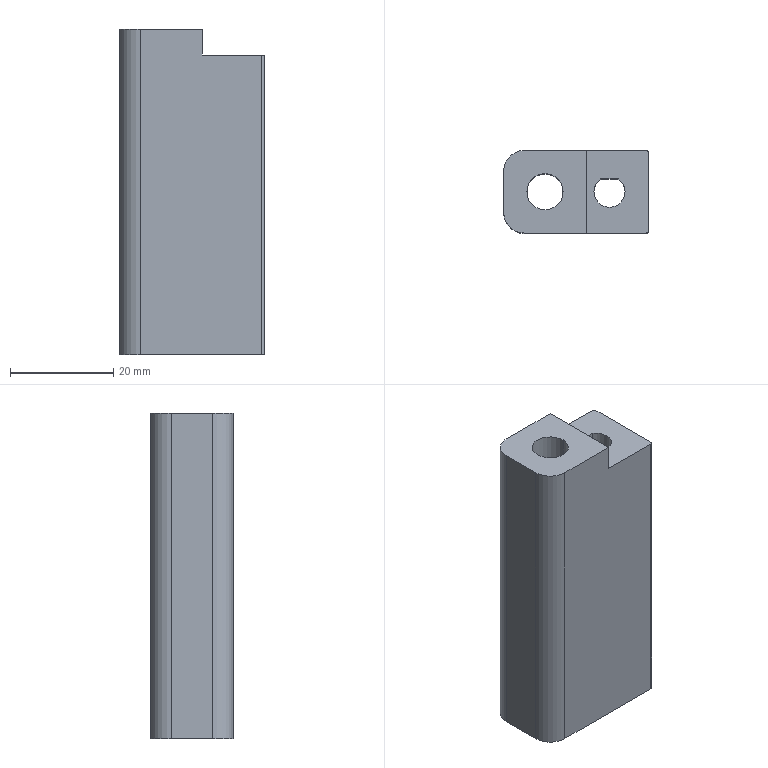Part | 1 solid | 19 faces | box 28 x 16 x 63 mm | volume 22260 mm3 | plane 10 | cylinder 9 | commonest cylinder face diameters 1 x2 7 x2 8 x2 11 x2 6 x1
STEP:
#1=CARTESIAN_POINT('',(0.,0.,0.));
#2=DIRECTION('',(0.,0.,1.));
#3=DIRECTION('',(1.,0.,0.));
#4=AXIS2_PLACEMENT_3D('',#1,#2,#3);
#5=CARTESIAN_POINT('',(-264.863,475.5,-113.051));
#6=VERTEX_POINT('',#5);
#7=CARTESIAN_POINT('',(-271.863,475.5,-113.051));
#8=VERTEX_POINT('',#7);
#9=CARTESIAN_POINT('',(-268.363,475.5,-113.051));
#10=DIRECTION('',(0.,0.,1.));
#11=DIRECTION('',(-1.,0.,0.));
#12=AXIS2_PLACEMENT_3D('',#9,#10,#11);
#13=CIRCLE('',#12,3.5);
#14=CARTESIAN_POINT('',(-248.863,468.,-113.051));
#15=DIRECTION('',(0.,0.,-1.));
#16=DIRECTION('',(1.,0.,0.));
#17=AXIS2_PLACEMENT_3D('',#14,#15,#16);
#18=PLANE('',#17);
#19=CARTESIAN_POINT('',(-23.,-7.5));
#20=CARTESIAN_POINT('',(-23.,-1.438));
#21=CARTESIAN_POINT('',(-17.75,-4.469));
#22=CARTESIAN_POINT('',(-12.5,-7.5));
#23=CARTESIAN_POINT('',(-17.75,-10.531));
#24=CARTESIAN_POINT('',(-23.,-13.562));
#25=CARTESIAN_POINT('',(-23.,-7.5));
#26=(BOUNDED_CURVE()B_SPLINE_CURVE(2,(#19,#20,#21,#22,#23,#24,#25),.UNSPECIFIED.,.T.,.F.)B_SPLINE_CURVE_WITH_KNOTS((1,2,2,2,2,1),(-2.094,0.,2.094,4.189,6.283,8.378),.UNSPECIFIED.)CURVE()GEOMETRIC_REPRESENTATION_ITEM()RATIONAL_B_SPLINE_CURVE((1.,0.5,1.,0.5,1.,0.5,1.))REPRESENTATION_ITEM(''));
#27=(GEOMETRIC_REPRESENTATION_CONTEXT(2)PARAMETRIC_REPRESENTATION_CONTEXT()REPRESENTATION_CONTEXT('',''));
#28=DEFINITIONAL_REPRESENTATION('',(#26),#27);
#29=PCURVE('',#18,#28);
#30=CARTESIAN_POINT('',(-268.363,475.5,-149.051));
#31=DIRECTION('',(0.,0.,1.));
#32=DIRECTION('',(0.,-1.,0.));
#33=AXIS2_PLACEMENT_3D('',#30,#31,#32);
#34=CYLINDRICAL_SURFACE('',#33,3.5);
#35=CARTESIAN_POINT('',(-1.571,36.));
#36=DIRECTION('',(1.,0.));
#37=VECTOR('',#36,1.);
#38=LINE('',#35,#37);
#39=(GEOMETRIC_REPRESENTATION_CONTEXT(2)PARAMETRIC_REPRESENTATION_CONTEXT()REPRESENTATION_CONTEXT('',''));
#40=DEFINITIONAL_REPRESENTATION('',(#38),#39);
#41=PCURVE('',#34,#40);
#42=SURFACE_CURVE('',#13,(#29,#41),.PCURVE_S1.);
#43=EDGE_CURVE('',#6,#8,#42,.T.);
#44=ORIENTED_EDGE('',*,*,#43,.F.);
#45=CARTESIAN_POINT('',(-268.363,475.5,-113.051));
#46=DIRECTION('',(0.,0.,1.));
#47=DIRECTION('',(-1.,0.,0.));
#48=AXIS2_PLACEMENT_3D('',#45,#46,#47);
#49=CIRCLE('',#48,3.5);
#50=CARTESIAN_POINT('',(-23.,-7.5));
#51=CARTESIAN_POINT('',(-23.,-1.438));
#52=CARTESIAN_POINT('',(-17.75,-4.469));
#53=CARTESIAN_POINT('',(-12.5,-7.5));
#54=CARTESIAN_POINT('',(-17.75,-10.531));
#55=CARTESIAN_POINT('',(-23.,-13.562));
#56=CARTESIAN_POINT('',(-23.,-7.5));
#57=(BOUNDED_CURVE()B_SPLINE_CURVE(2,(#50,#51,#52,#53,#54,#55,#56),.UNSPECIFIED.,.T.,.F.)B_SPLINE_CURVE_WITH_KNOTS((1,2,2,2,2,1),(-2.094,0.,2.094,4.189,6.283,8.378),.UNSPECIFIED.)CURVE()GEOMETRIC_REPRESENTATION_ITEM()RATIONAL_B_SPLINE_CURVE((1.,0.5,1.,0.5,1.,0.5,1.))REPRESENTATION_ITEM(''));
#58=(GEOMETRIC_REPRESENTATION_CONTEXT(2)PARAMETRIC_REPRESENTATION_CONTEXT()REPRESENTATION_CONTEXT('',''));
#59=DEFINITIONAL_REPRESENTATION('',(#57),#58);
#60=PCURVE('',#18,#59);
#61=CARTESIAN_POINT('',(-268.363,475.5,-149.051));
#62=DIRECTION('',(0.,0.,1.));
#63=DIRECTION('',(0.,1.,0.));
#64=AXIS2_PLACEMENT_3D('',#61,#62,#63);
#65=CYLINDRICAL_SURFACE('',#64,3.5);
#66=CARTESIAN_POINT('',(1.571,36.));
#67=DIRECTION('',(1.,0.));
#68=VECTOR('',#67,1.);
#69=LINE('',#66,#68);
#70=(GEOMETRIC_REPRESENTATION_CONTEXT(2)PARAMETRIC_REPRESENTATION_CONTEXT()REPRESENTATION_CONTEXT('',''));
#71=DEFINITIONAL_REPRESENTATION('',(#69),#70);
#72=PCURVE('',#65,#71);
#73=SURFACE_CURVE('',#49,(#60,#72),.PCURVE_S1.);
#74=EDGE_CURVE('',#8,#6,#73,.T.);
#75=ORIENTED_EDGE('',*,*,#74,.F.);
#76=EDGE_LOOP('',(#44,#75));
#77=FACE_BOUND('',#76,.T.);
#78=CARTESIAN_POINT('',(-260.363,483.5,-113.051));
#79=VERTEX_POINT('',#78);
#80=CARTESIAN_POINT('',(-260.363,467.5,-113.051));
#81=VERTEX_POINT('',#80);
#82=CARTESIAN_POINT('',(-260.363,468.,-113.051));
#83=DIRECTION('',(0.,-1.,0.));
#84=VECTOR('',#83,1.);
#85=LINE('',#82,#84);
#86=CARTESIAN_POINT('',(-11.5,0.));
#87=DIRECTION('',(0.,1.));
#88=VECTOR('',#87,1.);
#89=LINE('',#86,#88);
#90=(GEOMETRIC_REPRESENTATION_CONTEXT(2)PARAMETRIC_REPRESENTATION_CONTEXT()REPRESENTATION_CONTEXT('',''));
#91=DEFINITIONAL_REPRESENTATION('',(#89),#90);
#92=PCURVE('',#18,#91);
#93=CARTESIAN_POINT('',(-260.363,483.,-108.051));
#94=DIRECTION('',(1.,0.,0.));
#95=DIRECTION('',(0.,0.,1.));
#96=AXIS2_PLACEMENT_3D('',#93,#94,#95);
#97=PLANE('',#96);
#98=CARTESIAN_POINT('',(-5.,15.));
#99=DIRECTION('',(0.,1.));
#100=VECTOR('',#99,1.);
#101=LINE('',#98,#100);
#102=(GEOMETRIC_REPRESENTATION_CONTEXT(2)PARAMETRIC_REPRESENTATION_CONTEXT()REPRESENTATION_CONTEXT('',''));
#103=DEFINITIONAL_REPRESENTATION('',(#101),#102);
#104=PCURVE('',#97,#103);
#105=SURFACE_CURVE('',#85,(#92,#104),.PCURVE_S1.);
#106=EDGE_CURVE('',#79,#81,#105,.T.);
#107=ORIENTED_EDGE('',*,*,#106,.F.);
#108=CARTESIAN_POINT('',(-272.363,483.5,-113.051));
#109=VERTEX_POINT('',#108);
#110=CARTESIAN_POINT('',(-272.363,483.5,-113.051));
#111=DIRECTION('',(1.,0.,0.));
#112=VECTOR('',#111,1.);
#113=LINE('',#110,#112);
#114=CARTESIAN_POINT('',(-23.5,-15.5));
#115=DIRECTION('',(1.,0.));
#116=VECTOR('',#115,1.);
#117=LINE('',#114,#116);
#118=(GEOMETRIC_REPRESENTATION_CONTEXT(2)PARAMETRIC_REPRESENTATION_CONTEXT()REPRESENTATION_CONTEXT('',''));
#119=DEFINITIONAL_REPRESENTATION('',(#117),#118);
#120=PCURVE('',#18,#119);
#121=CARTESIAN_POINT('',(-272.363,483.5,-149.051));
#122=DIRECTION('',(0.,-1.,0.));
#123=DIRECTION('',(-1.,0.,0.));
#124=AXIS2_PLACEMENT_3D('',#121,#122,#123);
#125=PLANE('',#124);
#126=CARTESIAN_POINT('',(0.,-36.));
#127=DIRECTION('',(-1.,0.));
#128=VECTOR('',#127,1.);
#129=LINE('',#126,#128);
#130=(GEOMETRIC_REPRESENTATION_CONTEXT(2)PARAMETRIC_REPRESENTATION_CONTEXT()REPRESENTATION_CONTEXT('',''));
#131=DEFINITIONAL_REPRESENTATION('',(#129),#130);
#132=PCURVE('',#125,#131);
#133=SURFACE_CURVE('',#113,(#120,#132),.PCURVE_S1.);
#134=EDGE_CURVE('',#109,#79,#133,.T.);
#135=ORIENTED_EDGE('',*,*,#134,.F.);
#136=CARTESIAN_POINT('',(-276.363,479.5,-113.051));
#137=VERTEX_POINT('',#136);
#138=CARTESIAN_POINT('',(-272.363,479.5,-113.051));
#139=DIRECTION('',(0.,0.,-1.));
#140=DIRECTION('',(1.,0.,0.));
#141=AXIS2_PLACEMENT_3D('',#138,#139,#140);
#142=CIRCLE('',#141,4.);
#143=CARTESIAN_POINT('',(-23.5,-11.5));
#144=DIRECTION('',(1.,0.));
#145=AXIS2_PLACEMENT_2D('',#143,#144);
#146=CIRCLE('',#145,4.);
#147=(GEOMETRIC_REPRESENTATION_CONTEXT(2)PARAMETRIC_REPRESENTATION_CONTEXT()REPRESENTATION_CONTEXT('',''));
#148=DEFINITIONAL_REPRESENTATION('',(#146),#147);
#149=PCURVE('',#18,#148);
#150=CARTESIAN_POINT('',(-272.363,479.5,-149.051));
#151=DIRECTION('',(0.,0.,1.));
#152=DIRECTION('',(0.7071,-0.7071,0.));
#153=AXIS2_PLACEMENT_3D('',#150,#151,#152);
#154=CYLINDRICAL_SURFACE('',#153,4.);
#155=CARTESIAN_POINT('',(7.069,36.));
#156=DIRECTION('',(-1.,0.));
#157=VECTOR('',#156,1.);
#158=LINE('',#155,#157);
#159=(GEOMETRIC_REPRESENTATION_CONTEXT(2)PARAMETRIC_REPRESENTATION_CONTEXT()REPRESENTATION_CONTEXT('',''));
#160=DEFINITIONAL_REPRESENTATION('',(#158),#159);
#161=PCURVE('',#154,#160);
#162=SURFACE_CURVE('',#142,(#149,#161),.PCURVE_S1.);
#163=EDGE_CURVE('',#137,#109,#162,.T.);
#164=ORIENTED_EDGE('',*,*,#163,.F.);
#165=CARTESIAN_POINT('',(-276.363,471.5,-113.051));
#166=VERTEX_POINT('',#165);
#167=CARTESIAN_POINT('',(-276.363,471.5,-113.051));
#168=DIRECTION('',(0.,1.,0.));
#169=VECTOR('',#168,1.);
#170=LINE('',#167,#169);
#171=CARTESIAN_POINT('',(-27.5,-3.5));
#172=DIRECTION('',(0.,-1.));
#173=VECTOR('',#172,1.);
#174=LINE('',#171,#173);
#175=(GEOMETRIC_REPRESENTATION_CONTEXT(2)PARAMETRIC_REPRESENTATION_CONTEXT()REPRESENTATION_CONTEXT('',''));
#176=DEFINITIONAL_REPRESENTATION('',(#174),#175);
#177=PCURVE('',#18,#176);
#178=CARTESIAN_POINT('',(-276.363,471.5,-149.051));
#179=DIRECTION('',(1.,0.,0.));
#180=DIRECTION('',(0.,-1.,0.));
#181=AXIS2_PLACEMENT_3D('',#178,#179,#180);
#182=PLANE('',#181);
#183=CARTESIAN_POINT('',(0.,-36.));
#184=DIRECTION('',(-1.,0.));
#185=VECTOR('',#184,1.);
#186=LINE('',#183,#185);
#187=(GEOMETRIC_REPRESENTATION_CONTEXT(2)PARAMETRIC_REPRESENTATION_CONTEXT()REPRESENTATION_CONTEXT('',''));
#188=DEFINITIONAL_REPRESENTATION('',(#186),#187);
#189=PCURVE('',#182,#188);
#190=SURFACE_CURVE('',#170,(#177,#189),.PCURVE_S1.);
#191=EDGE_CURVE('',#166,#137,#190,.T.);
#192=ORIENTED_EDGE('',*,*,#191,.F.);
#193=CARTESIAN_POINT('',(-272.363,467.5,-113.051));
#194=VERTEX_POINT('',#193);
#195=CARTESIAN_POINT('',(-272.363,471.5,-113.051));
#196=DIRECTION('',(0.,0.,-1.));
#197=DIRECTION('',(1.,0.,0.));
#198=AXIS2_PLACEMENT_3D('',#195,#196,#197);
#199=CIRCLE('',#198,4.);
#200=CARTESIAN_POINT('',(-23.5,-3.5));
#201=DIRECTION('',(1.,0.));
#202=AXIS2_PLACEMENT_2D('',#200,#201);
#203=CIRCLE('',#202,4.);
#204=(GEOMETRIC_REPRESENTATION_CONTEXT(2)PARAMETRIC_REPRESENTATION_CONTEXT()REPRESENTATION_CONTEXT('',''));
#205=DEFINITIONAL_REPRESENTATION('',(#203),#204);
#206=PCURVE('',#18,#205);
#207=CARTESIAN_POINT('',(-272.363,471.5,-149.051));
#208=DIRECTION('',(0.,0.,1.));
#209=DIRECTION('',(0.7071,0.7071,0.));
#210=AXIS2_PLACEMENT_3D('',#207,#208,#209);
#211=CYLINDRICAL_SURFACE('',#210,4.);
#212=CARTESIAN_POINT('',(5.498,36.));
#213=DIRECTION('',(-1.,0.));
#214=VECTOR('',#213,1.);
#215=LINE('',#212,#214);
#216=(GEOMETRIC_REPRESENTATION_CONTEXT(2)PARAMETRIC_REPRESENTATION_CONTEXT()REPRESENTATION_CONTEXT('',''));
#217=DEFINITIONAL_REPRESENTATION('',(#215),#216);
#218=PCURVE('',#211,#217);
#219=SURFACE_CURVE('',#199,(#206,#218),.PCURVE_S1.);
#220=EDGE_CURVE('',#194,#166,#219,.T.);
#221=ORIENTED_EDGE('',*,*,#220,.F.);
#222=CARTESIAN_POINT('',(-248.863,467.5,-113.051));
#223=DIRECTION('',(-1.,0.,0.));
#224=VECTOR('',#223,1.);
#225=LINE('',#222,#224);
#226=CARTESIAN_POINT('',(0.,0.5));
#227=DIRECTION('',(-1.,0.));
#228=VECTOR('',#227,1.);
#229=LINE('',#226,#228);
#230=(GEOMETRIC_REPRESENTATION_CONTEXT(2)PARAMETRIC_REPRESENTATION_CONTEXT()REPRESENTATION_CONTEXT('',''));
#231=DEFINITIONAL_REPRESENTATION('',(#229),#230);
#232=PCURVE('',#18,#231);
#233=CARTESIAN_POINT('',(-248.863,467.5,-149.051));
#234=DIRECTION('',(0.,1.,0.));
#235=DIRECTION('',(0.,0.,-1.));
#236=AXIS2_PLACEMENT_3D('',#233,#234,#235);
#237=PLANE('',#236);
#238=CARTESIAN_POINT('',(-36.,0.));
#239=DIRECTION('',(0.,1.));
#240=VECTOR('',#239,1.);
#241=LINE('',#238,#240);
#242=(GEOMETRIC_REPRESENTATION_CONTEXT(2)PARAMETRIC_REPRESENTATION_CONTEXT()REPRESENTATION_CONTEXT('',''));
#243=DEFINITIONAL_REPRESENTATION('',(#241),#242);
#244=PCURVE('',#237,#243);
#245=SURFACE_CURVE('',#225,(#232,#244),.PCURVE_S1.);
#246=EDGE_CURVE('',#81,#194,#245,.T.);
#247=ORIENTED_EDGE('',*,*,#246,.F.);
#248=EDGE_LOOP('',(#107,#135,#164,#192,#221,#247));
#249=FACE_BOUND('',#248,.T.);
#250=ADVANCED_FACE('',(#77,#249),#18,.F.);
#251=CARTESIAN_POINT('',(-248.863,467.5,-176.051));
#252=VERTEX_POINT('',#251);
#253=CARTESIAN_POINT('',(-248.863,467.5,-118.051));
#254=VERTEX_POINT('',#253);
#255=CARTESIAN_POINT('',(-248.863,467.5,-149.051));
#256=DIRECTION('',(0.,0.,1.));
#257=VECTOR('',#256,1.);
#258=LINE('',#255,#257);
#259=CARTESIAN_POINT('',(0.,0.));
#260=DIRECTION('',(-1.,0.));
#261=VECTOR('',#260,1.);
#262=LINE('',#259,#261);
#263=(GEOMETRIC_REPRESENTATION_CONTEXT(2)PARAMETRIC_REPRESENTATION_CONTEXT()REPRESENTATION_CONTEXT('',''));
#264=DEFINITIONAL_REPRESENTATION('',(#262),#263);
#265=PCURVE('',#237,#264);
#266=CARTESIAN_POINT('',(-248.863,468.,-149.051));
#267=DIRECTION('',(0.,0.,1.));
#268=DIRECTION('',(-0.7071,0.7071,0.));
#269=AXIS2_PLACEMENT_3D('',#266,#267,#268);
#270=CYLINDRICAL_SURFACE('',#269,0.5);
#271=CARTESIAN_POINT('',(2.356,0.));
#272=DIRECTION('',(0.,1.));
#273=VECTOR('',#272,1.);
#274=LINE('',#271,#273);
#275=(GEOMETRIC_REPRESENTATION_CONTEXT(2)PARAMETRIC_REPRESENTATION_CONTEXT()REPRESENTATION_CONTEXT('',''));
#276=DEFINITIONAL_REPRESENTATION('',(#274),#275);
#277=PCURVE('',#270,#276);
#278=SURFACE_CURVE('',#258,(#265,#277),.PCURVE_S1.);
#279=EDGE_CURVE('',#252,#254,#278,.T.);
#280=ORIENTED_EDGE('',*,*,#279,.T.);
#281=CARTESIAN_POINT('',(-260.363,467.5,-118.051));
#282=VERTEX_POINT('',#281);
#283=CARTESIAN_POINT('',(-248.863,467.5,-118.051));
#284=DIRECTION('',(-1.,0.,0.));
#285=VECTOR('',#284,1.);
#286=LINE('',#283,#285);
#287=CARTESIAN_POINT('',(-31.,0.));
#288=DIRECTION('',(0.,1.));
#289=VECTOR('',#288,1.);
#290=LINE('',#287,#289);
#291=(GEOMETRIC_REPRESENTATION_CONTEXT(2)PARAMETRIC_REPRESENTATION_CONTEXT()REPRESENTATION_CONTEXT('',''));
#292=DEFINITIONAL_REPRESENTATION('',(#290),#291);
#293=PCURVE('',#237,#292);
#294=CARTESIAN_POINT('',(-254.382,475.5,-118.051));
#295=DIRECTION('',(0.,0.,-1.));
#296=DIRECTION('',(1.,0.,0.));
#297=AXIS2_PLACEMENT_3D('',#294,#295,#296);
#298=PLANE('',#297);
#299=CARTESIAN_POINT('',(5.519,8.));
#300=DIRECTION('',(-1.,0.));
#301=VECTOR('',#300,1.);
#302=LINE('',#299,#301);
#303=(GEOMETRIC_REPRESENTATION_CONTEXT(2)PARAMETRIC_REPRESENTATION_CONTEXT()REPRESENTATION_CONTEXT('',''));
#304=DEFINITIONAL_REPRESENTATION('',(#302),#303);
#305=PCURVE('',#298,#304);
#306=SURFACE_CURVE('',#286,(#293,#305),.PCURVE_S1.);
#307=EDGE_CURVE('',#254,#282,#306,.T.);
#308=ORIENTED_EDGE('',*,*,#307,.T.);
#309=CARTESIAN_POINT('',(-260.363,467.5,-149.051));
#310=DIRECTION('',(0.,0.,-1.));
#311=VECTOR('',#310,1.);
#312=LINE('',#309,#311);
#313=CARTESIAN_POINT('',(0.,11.5));
#314=DIRECTION('',(1.,0.));
#315=VECTOR('',#314,1.);
#316=LINE('',#313,#315);
#317=(GEOMETRIC_REPRESENTATION_CONTEXT(2)PARAMETRIC_REPRESENTATION_CONTEXT()REPRESENTATION_CONTEXT('',''));
#318=DEFINITIONAL_REPRESENTATION('',(#316),#317);
#319=PCURVE('',#237,#318);
#320=CARTESIAN_POINT('',(-41.,15.5));
#321=DIRECTION('',(-1.,0.));
#322=VECTOR('',#321,1.);
#323=LINE('',#320,#322);
#324=(GEOMETRIC_REPRESENTATION_CONTEXT(2)PARAMETRIC_REPRESENTATION_CONTEXT()REPRESENTATION_CONTEXT('',''));
#325=DEFINITIONAL_REPRESENTATION('',(#323),#324);
#326=PCURVE('',#97,#325);
#327=SURFACE_CURVE('',#312,(#319,#326),.PCURVE_S1.);
#328=EDGE_CURVE('',#81,#282,#327,.T.);
#329=ORIENTED_EDGE('',*,*,#328,.F.);
#330=ORIENTED_EDGE('',*,*,#246,.T.);
#331=CARTESIAN_POINT('',(-272.363,467.5,-176.051));
#332=VERTEX_POINT('',#331);
#333=CARTESIAN_POINT('',(-272.363,467.5,-149.051));
#334=DIRECTION('',(0.,0.,1.));
#335=VECTOR('',#334,1.);
#336=LINE('',#333,#335);
#337=CARTESIAN_POINT('',(0.,23.5));
#338=DIRECTION('',(-1.,0.));
#339=VECTOR('',#338,1.);
#340=LINE('',#337,#339);
#341=(GEOMETRIC_REPRESENTATION_CONTEXT(2)PARAMETRIC_REPRESENTATION_CONTEXT()REPRESENTATION_CONTEXT('',''));
#342=DEFINITIONAL_REPRESENTATION('',(#340),#341);
#343=PCURVE('',#237,#342);
#344=CARTESIAN_POINT('',(3.927,0.));
#345=DIRECTION('',(0.,1.));
#346=VECTOR('',#345,1.);
#347=LINE('',#344,#346);
#348=(GEOMETRIC_REPRESENTATION_CONTEXT(2)PARAMETRIC_REPRESENTATION_CONTEXT()REPRESENTATION_CONTEXT('',''));
#349=DEFINITIONAL_REPRESENTATION('',(#347),#348);
#350=PCURVE('',#211,#349);
#351=SURFACE_CURVE('',#336,(#343,#350),.PCURVE_S1.);
#352=EDGE_CURVE('',#332,#194,#351,.T.);
#353=ORIENTED_EDGE('',*,*,#352,.F.);
#354=CARTESIAN_POINT('',(-248.863,467.5,-176.051));
#355=DIRECTION('',(-1.,0.,0.));
#356=VECTOR('',#355,1.);
#357=LINE('',#354,#356);
#358=CARTESIAN_POINT('',(27.,0.));
#359=DIRECTION('',(0.,1.));
#360=VECTOR('',#359,1.);
#361=LINE('',#358,#360);
#362=(GEOMETRIC_REPRESENTATION_CONTEXT(2)PARAMETRIC_REPRESENTATION_CONTEXT()REPRESENTATION_CONTEXT('',''));
#363=DEFINITIONAL_REPRESENTATION('',(#361),#362);
#364=PCURVE('',#237,#363);
#365=CARTESIAN_POINT('',(-248.863,468.,-176.051));
#366=DIRECTION('',(0.,0.,-1.));
#367=DIRECTION('',(1.,0.,0.));
#368=AXIS2_PLACEMENT_3D('',#365,#366,#367);
#369=PLANE('',#368);
#370=CARTESIAN_POINT('',(0.,0.5));
#371=DIRECTION('',(-1.,0.));
#372=VECTOR('',#371,1.);
#373=LINE('',#370,#372);
#374=(GEOMETRIC_REPRESENTATION_CONTEXT(2)PARAMETRIC_REPRESENTATION_CONTEXT()REPRESENTATION_CONTEXT('',''));
#375=DEFINITIONAL_REPRESENTATION('',(#373),#374);
#376=PCURVE('',#369,#375);
#377=SURFACE_CURVE('',#357,(#364,#376),.PCURVE_S1.);
#378=EDGE_CURVE('',#252,#332,#377,.T.);
#379=ORIENTED_EDGE('',*,*,#378,.F.);
#380=EDGE_LOOP('',(#280,#308,#329,#330,#353,#379));
#381=FACE_BOUND('',#380,.T.);
#382=ADVANCED_FACE('',(#381),#237,.F.);
#383=CARTESIAN_POINT('',(-248.363,483.,-176.051));
#384=VERTEX_POINT('',#383);
#385=CARTESIAN_POINT('',(-248.363,468.,-176.051));
#386=VERTEX_POINT('',#385);
#387=CARTESIAN_POINT('',(-248.363,483.,-176.051));
#388=DIRECTION('',(0.,-1.,0.));
#389=VECTOR('',#388,1.);
#390=LINE('',#387,#389);
#391=CARTESIAN_POINT('',(0.5,-15.));
#392=DIRECTION('',(0.,1.));
#393=VECTOR('',#392,1.);
#394=LINE('',#391,#393);
#395=(GEOMETRIC_REPRESENTATION_CONTEXT(2)PARAMETRIC_REPRESENTATION_CONTEXT()REPRESENTATION_CONTEXT('',''));
#396=DEFINITIONAL_REPRESENTATION('',(#394),#395);
#397=PCURVE('',#369,#396);
#398=CARTESIAN_POINT('',(-248.363,483.,-149.051));
#399=DIRECTION('',(-1.,0.,0.));
#400=DIRECTION('',(0.,0.,-1.));
#401=AXIS2_PLACEMENT_3D('',#398,#399,#400);
#402=PLANE('',#401);
#403=CARTESIAN_POINT('',(27.,0.));
#404=DIRECTION('',(0.,1.));
#405=VECTOR('',#404,1.);
#406=LINE('',#403,#405);
#407=(GEOMETRIC_REPRESENTATION_CONTEXT(2)PARAMETRIC_REPRESENTATION_CONTEXT()REPRESENTATION_CONTEXT('',''));
#408=DEFINITIONAL_REPRESENTATION('',(#406),#407);
#409=PCURVE('',#402,#408);
#410=SURFACE_CURVE('',#390,(#397,#409),.PCURVE_S1.);
#411=EDGE_CURVE('',#384,#386,#410,.T.);
#412=ORIENTED_EDGE('',*,*,#411,.T.);
#413=CARTESIAN_POINT('',(-248.863,468.,-176.051));
#414=DIRECTION('',(0.,0.,-1.));
#415=DIRECTION('',(-1.,0.,0.));
#416=AXIS2_PLACEMENT_3D('',#413,#414,#415);
#417=CIRCLE('',#416,0.5);
#418=CARTESIAN_POINT('',(0.,0.));
#419=DIRECTION('',(-1.,0.));
#420=AXIS2_PLACEMENT_2D('',#418,#419);
#421=CIRCLE('',#420,0.5);
#422=(GEOMETRIC_REPRESENTATION_CONTEXT(2)PARAMETRIC_REPRESENTATION_CONTEXT()REPRESENTATION_CONTEXT('',''));
#423=DEFINITIONAL_REPRESENTATION('',(#421),#422);
#424=PCURVE('',#369,#423);
#425=CARTESIAN_POINT('',(7.069,-27.));
#426=DIRECTION('',(-1.,0.));
#427=VECTOR('',#426,1.);
#428=LINE('',#425,#427);
#429=(GEOMETRIC_REPRESENTATION_CONTEXT(2)PARAMETRIC_REPRESENTATION_CONTEXT()REPRESENTATION_CONTEXT('',''));
#430=DEFINITIONAL_REPRESENTATION('',(#428),#429);
#431=PCURVE('',#270,#430);
#432=SURFACE_CURVE('',#417,(#424,#431),.PCURVE_S1.);
#433=EDGE_CURVE('',#386,#252,#432,.T.);
#434=ORIENTED_EDGE('',*,*,#433,.T.);
#435=ORIENTED_EDGE('',*,*,#378,.T.);
#436=CARTESIAN_POINT('',(-276.363,471.5,-176.051));
#437=VERTEX_POINT('',#436);
#438=CARTESIAN_POINT('',(-272.363,471.5,-176.051));
#439=DIRECTION('',(0.,0.,-1.));
#440=DIRECTION('',(-1.,0.,0.));
#441=AXIS2_PLACEMENT_3D('',#438,#439,#440);
#442=CIRCLE('',#441,4.);
#443=CARTESIAN_POINT('',(-23.5,-3.5));
#444=DIRECTION('',(-1.,0.));
#445=AXIS2_PLACEMENT_2D('',#443,#444);
#446=CIRCLE('',#445,4.);
#447=(GEOMETRIC_REPRESENTATION_CONTEXT(2)PARAMETRIC_REPRESENTATION_CONTEXT()REPRESENTATION_CONTEXT('',''));
#448=DEFINITIONAL_REPRESENTATION('',(#446),#447);
#449=PCURVE('',#369,#448);
#450=CARTESIAN_POINT('',(8.639,-27.));
#451=DIRECTION('',(-1.,0.));
#452=VECTOR('',#451,1.);
#453=LINE('',#450,#452);
#454=(GEOMETRIC_REPRESENTATION_CONTEXT(2)PARAMETRIC_REPRESENTATION_CONTEXT()REPRESENTATION_CONTEXT('',''));
#455=DEFINITIONAL_REPRESENTATION('',(#453),#454);
#456=PCURVE('',#211,#455);
#457=SURFACE_CURVE('',#442,(#449,#456),.PCURVE_S1.);
#458=EDGE_CURVE('',#332,#437,#457,.T.);
#459=ORIENTED_EDGE('',*,*,#458,.T.);
#460=CARTESIAN_POINT('',(-276.363,479.5,-176.051));
#461=VERTEX_POINT('',#460);
#462=CARTESIAN_POINT('',(-276.363,471.5,-176.051));
#463=DIRECTION('',(0.,1.,0.));
#464=VECTOR('',#463,1.);
#465=LINE('',#462,#464);
#466=CARTESIAN_POINT('',(-27.5,-3.5));
#467=DIRECTION('',(0.,-1.));
#468=VECTOR('',#467,1.);
#469=LINE('',#466,#468);
#470=(GEOMETRIC_REPRESENTATION_CONTEXT(2)PARAMETRIC_REPRESENTATION_CONTEXT()REPRESENTATION_CONTEXT('',''));
#471=DEFINITIONAL_REPRESENTATION('',(#469),#470);
#472=PCURVE('',#369,#471);
#473=CARTESIAN_POINT('',(0.,27.));
#474=DIRECTION('',(-1.,0.));
#475=VECTOR('',#474,1.);
#476=LINE('',#473,#475);
#477=(GEOMETRIC_REPRESENTATION_CONTEXT(2)PARAMETRIC_REPRESENTATION_CONTEXT()REPRESENTATION_CONTEXT('',''));
#478=DEFINITIONAL_REPRESENTATION('',(#476),#477);
#479=PCURVE('',#182,#478);
#480=SURFACE_CURVE('',#465,(#472,#479),.PCURVE_S1.);
#481=EDGE_CURVE('',#437,#461,#480,.T.);
#482=ORIENTED_EDGE('',*,*,#481,.T.);
#483=CARTESIAN_POINT('',(-272.363,483.5,-176.051));
#484=VERTEX_POINT('',#483);
#485=CARTESIAN_POINT('',(-272.363,479.5,-176.051));
#486=DIRECTION('',(0.,0.,-1.));
#487=DIRECTION('',(-1.,0.,0.));
#488=AXIS2_PLACEMENT_3D('',#485,#486,#487);
#489=CIRCLE('',#488,4.);
#490=CARTESIAN_POINT('',(-23.5,-11.5));
#491=DIRECTION('',(-1.,0.));
#492=AXIS2_PLACEMENT_2D('',#490,#491);
#493=CIRCLE('',#492,4.);
#494=(GEOMETRIC_REPRESENTATION_CONTEXT(2)PARAMETRIC_REPRESENTATION_CONTEXT()REPRESENTATION_CONTEXT('',''));
#495=DEFINITIONAL_REPRESENTATION('',(#493),#494);
#496=PCURVE('',#369,#495);
#497=CARTESIAN_POINT('',(3.927,-27.));
#498=DIRECTION('',(-1.,0.));
#499=VECTOR('',#498,1.);
#500=LINE('',#497,#499);
#501=(GEOMETRIC_REPRESENTATION_CONTEXT(2)PARAMETRIC_REPRESENTATION_CONTEXT()REPRESENTATION_CONTEXT('',''));
#502=DEFINITIONAL_REPRESENTATION('',(#500),#501);
#503=PCURVE('',#154,#502);
#504=SURFACE_CURVE('',#489,(#496,#503),.PCURVE_S1.);
#505=EDGE_CURVE('',#461,#484,#504,.T.);
#506=ORIENTED_EDGE('',*,*,#505,.T.);
#507=CARTESIAN_POINT('',(-248.863,483.5,-176.051));
#508=VERTEX_POINT('',#507);
#509=CARTESIAN_POINT('',(-272.363,483.5,-176.051));
#510=DIRECTION('',(1.,0.,0.));
#511=VECTOR('',#510,1.);
#512=LINE('',#509,#511);
#513=CARTESIAN_POINT('',(-23.5,-15.5));
#514=DIRECTION('',(1.,0.));
#515=VECTOR('',#514,1.);
#516=LINE('',#513,#515);
#517=(GEOMETRIC_REPRESENTATION_CONTEXT(2)PARAMETRIC_REPRESENTATION_CONTEXT()REPRESENTATION_CONTEXT('',''));
#518=DEFINITIONAL_REPRESENTATION('',(#516),#517);
#519=PCURVE('',#369,#518);
#520=CARTESIAN_POINT('',(0.,27.));
#521=DIRECTION('',(-1.,0.));
#522=VECTOR('',#521,1.);
#523=LINE('',#520,#522);
#524=(GEOMETRIC_REPRESENTATION_CONTEXT(2)PARAMETRIC_REPRESENTATION_CONTEXT()REPRESENTATION_CONTEXT('',''));
#525=DEFINITIONAL_REPRESENTATION('',(#523),#524);
#526=PCURVE('',#125,#525);
#527=SURFACE_CURVE('',#512,(#519,#526),.PCURVE_S1.);
#528=EDGE_CURVE('',#484,#508,#527,.T.);
#529=ORIENTED_EDGE('',*,*,#528,.T.);
#530=CARTESIAN_POINT('',(-248.863,483.,-176.051));
#531=DIRECTION('',(0.,0.,-1.));
#532=DIRECTION('',(-1.,0.,0.));
#533=AXIS2_PLACEMENT_3D('',#530,#531,#532);
#534=CIRCLE('',#533,0.5);
#535=CARTESIAN_POINT('',(0.,-15.));
#536=DIRECTION('',(-1.,0.));
#537=AXIS2_PLACEMENT_2D('',#535,#536);
#538=CIRCLE('',#537,0.5);
#539=(GEOMETRIC_REPRESENTATION_CONTEXT(2)PARAMETRIC_REPRESENTATION_CONTEXT()REPRESENTATION_CONTEXT('',''));
#540=DEFINITIONAL_REPRESENTATION('',(#538),#539);
#541=PCURVE('',#369,#540);
#542=CARTESIAN_POINT('',(-248.863,483.,-149.051));
#543=DIRECTION('',(0.,0.,1.));
#544=DIRECTION('',(-0.7071,-0.7071,0.));
#545=AXIS2_PLACEMENT_3D('',#542,#543,#544);
#546=CYLINDRICAL_SURFACE('',#545,0.5);
#547=CARTESIAN_POINT('',(5.498,-27.));
#548=DIRECTION('',(-1.,0.));
#549=VECTOR('',#548,1.);
#550=LINE('',#547,#549);
#551=(GEOMETRIC_REPRESENTATION_CONTEXT(2)PARAMETRIC_REPRESENTATION_CONTEXT()REPRESENTATION_CONTEXT('',''));
#552=DEFINITIONAL_REPRESENTATION('',(#550),#551);
#553=PCURVE('',#546,#552);
#554=SURFACE_CURVE('',#534,(#541,#553),.PCURVE_S1.);
#555=EDGE_CURVE('',#508,#384,#554,.T.);
#556=ORIENTED_EDGE('',*,*,#555,.T.);
#557=EDGE_LOOP('',(#412,#434,#435,#459,#482,#506,#529,#556));
#558=FACE_BOUND('',#557,.T.);
#559=CARTESIAN_POINT('',(-273.863,475.5,-176.051));
#560=VERTEX_POINT('',#559);
#561=CARTESIAN_POINT('',(-262.863,475.5,-176.051));
#562=VERTEX_POINT('',#561);
#563=CARTESIAN_POINT('',(-268.363,475.5,-176.051));
#564=DIRECTION('',(0.,0.,1.));
#565=DIRECTION('',(-1.,0.,0.));
#566=AXIS2_PLACEMENT_3D('',#563,#564,#565);
#567=CIRCLE('',#566,5.5);
#568=CARTESIAN_POINT('',(-25.,-7.5));
#569=CARTESIAN_POINT('',(-25.,2.026));
#570=CARTESIAN_POINT('',(-16.75,-2.737));
#571=CARTESIAN_POINT('',(-8.5,-7.5));
#572=CARTESIAN_POINT('',(-16.75,-12.263));
#573=CARTESIAN_POINT('',(-25.,-17.026));
#574=CARTESIAN_POINT('',(-25.,-7.5));
#575=(BOUNDED_CURVE()B_SPLINE_CURVE(2,(#568,#569,#570,#571,#572,#573,#574),.UNSPECIFIED.,.T.,.F.)B_SPLINE_CURVE_WITH_KNOTS((1,2,2,2,2,1),(-2.094,0.,2.094,4.189,6.283,8.378),.UNSPECIFIED.)CURVE()GEOMETRIC_REPRESENTATION_ITEM()RATIONAL_B_SPLINE_CURVE((1.,0.5,1.,0.5,1.,0.5,1.))REPRESENTATION_ITEM(''));
#576=(GEOMETRIC_REPRESENTATION_CONTEXT(2)PARAMETRIC_REPRESENTATION_CONTEXT()REPRESENTATION_CONTEXT('',''));
#577=DEFINITIONAL_REPRESENTATION('',(#575),#576);
#578=PCURVE('',#369,#577);
#579=CARTESIAN_POINT('',(-268.363,475.5,-149.051));
#580=DIRECTION('',(0.,0.,1.));
#581=DIRECTION('',(0.,1.,0.));
#582=AXIS2_PLACEMENT_3D('',#579,#580,#581);
#583=CYLINDRICAL_SURFACE('',#582,5.5);
#584=CARTESIAN_POINT('',(1.571,-27.));
#585=DIRECTION('',(1.,0.));
#586=VECTOR('',#585,1.);
#587=LINE('',#584,#586);
#588=(GEOMETRIC_REPRESENTATION_CONTEXT(2)PARAMETRIC_REPRESENTATION_CONTEXT()REPRESENTATION_CONTEXT('',''));
#589=DEFINITIONAL_REPRESENTATION('',(#587),#588);
#590=PCURVE('',#583,#589);
#591=SURFACE_CURVE('',#567,(#578,#590),.PCURVE_S1.);
#592=EDGE_CURVE('',#560,#562,#591,.T.);
#593=ORIENTED_EDGE('',*,*,#592,.T.);
#594=CARTESIAN_POINT('',(-268.363,475.5,-176.051));
#595=DIRECTION('',(0.,0.,1.));
#596=DIRECTION('',(-1.,0.,0.));
#597=AXIS2_PLACEMENT_3D('',#594,#595,#596);
#598=CIRCLE('',#597,5.5);
#599=CARTESIAN_POINT('',(-25.,-7.5));
#600=CARTESIAN_POINT('',(-25.,2.026));
#601=CARTESIAN_POINT('',(-16.75,-2.737));
#602=CARTESIAN_POINT('',(-8.5,-7.5));
#603=CARTESIAN_POINT('',(-16.75,-12.263));
#604=CARTESIAN_POINT('',(-25.,-17.026));
#605=CARTESIAN_POINT('',(-25.,-7.5));
#606=(BOUNDED_CURVE()B_SPLINE_CURVE(2,(#599,#600,#601,#602,#603,#604,#605),.UNSPECIFIED.,.T.,.F.)B_SPLINE_CURVE_WITH_KNOTS((1,2,2,2,2,1),(-2.094,0.,2.094,4.189,6.283,8.378),.UNSPECIFIED.)CURVE()GEOMETRIC_REPRESENTATION_ITEM()RATIONAL_B_SPLINE_CURVE((1.,0.5,1.,0.5,1.,0.5,1.))REPRESENTATION_ITEM(''));
#607=(GEOMETRIC_REPRESENTATION_CONTEXT(2)PARAMETRIC_REPRESENTATION_CONTEXT()REPRESENTATION_CONTEXT('',''));
#608=DEFINITIONAL_REPRESENTATION('',(#606),#607);
#609=PCURVE('',#369,#608);
#610=CARTESIAN_POINT('',(-268.363,475.5,-149.051));
#611=DIRECTION('',(0.,0.,1.));
#612=DIRECTION('',(0.,-1.,0.));
#613=AXIS2_PLACEMENT_3D('',#610,#611,#612);
#614=CYLINDRICAL_SURFACE('',#613,5.5);
#615=CARTESIAN_POINT('',(-1.571,-27.));
#616=DIRECTION('',(1.,0.));
#617=VECTOR('',#616,1.);
#618=LINE('',#615,#617);
#619=(GEOMETRIC_REPRESENTATION_CONTEXT(2)PARAMETRIC_REPRESENTATION_CONTEXT()REPRESENTATION_CONTEXT('',''));
#620=DEFINITIONAL_REPRESENTATION('',(#618),#619);
#621=PCURVE('',#614,#620);
#622=SURFACE_CURVE('',#598,(#609,#621),.PCURVE_S1.);
#623=EDGE_CURVE('',#562,#560,#622,.T.);
#624=ORIENTED_EDGE('',*,*,#623,.T.);
#625=EDGE_LOOP('',(#593,#624));
#626=FACE_BOUND('',#625,.T.);
#627=CARTESIAN_POINT('',(-257.54,478.,-176.051));
#628=VERTEX_POINT('',#627);
#629=CARTESIAN_POINT('',(-254.224,478.,-176.051));
#630=VERTEX_POINT('',#629);
#631=CARTESIAN_POINT('',(-255.882,475.5,-176.051));
#632=DIRECTION('',(0.,0.,1.));
#633=DIRECTION('',(-1.,0.,0.));
#634=AXIS2_PLACEMENT_3D('',#631,#632,#633);
#635=CIRCLE('',#634,3.);
#636=CARTESIAN_POINT('',(-10.019,-7.5));
#637=CARTESIAN_POINT('',(-10.019,-2.304));
#638=CARTESIAN_POINT('',(-5.519,-4.902));
#639=CARTESIAN_POINT('',(-1.019,-7.5));
#640=CARTESIAN_POINT('',(-5.519,-10.098));
#641=CARTESIAN_POINT('',(-10.019,-12.696));
#642=CARTESIAN_POINT('',(-10.019,-7.5));
#643=(BOUNDED_CURVE()B_SPLINE_CURVE(2,(#636,#637,#638,#639,#640,#641,#642),.UNSPECIFIED.,.T.,.F.)B_SPLINE_CURVE_WITH_KNOTS((1,2,2,2,2,1),(-2.094,0.,2.094,4.189,6.283,8.378),.UNSPECIFIED.)CURVE()GEOMETRIC_REPRESENTATION_ITEM()RATIONAL_B_SPLINE_CURVE((1.,0.5,1.,0.5,1.,0.5,1.))REPRESENTATION_ITEM(''));
#644=(GEOMETRIC_REPRESENTATION_CONTEXT(2)PARAMETRIC_REPRESENTATION_CONTEXT()REPRESENTATION_CONTEXT('',''));
#645=DEFINITIONAL_REPRESENTATION('',(#643),#644);
#646=PCURVE('',#369,#645);
#647=CARTESIAN_POINT('',(-255.882,475.5,-635.051));
#648=DIRECTION('',(0.,0.,1.));
#649=DIRECTION('',(0.,1.,0.));
#650=AXIS2_PLACEMENT_3D('',#647,#648,#649);
#651=CYLINDRICAL_SURFACE('',#650,3.);
#652=CARTESIAN_POINT('',(-4.712,459.));
#653=DIRECTION('',(1.,0.));
#654=VECTOR('',#653,1.);
#655=LINE('',#652,#654);
#656=(GEOMETRIC_REPRESENTATION_CONTEXT(2)PARAMETRIC_REPRESENTATION_CONTEXT()REPRESENTATION_CONTEXT('',''));
#657=DEFINITIONAL_REPRESENTATION('',(#655),#656);
#658=PCURVE('',#651,#657);
#659=SURFACE_CURVE('',#635,(#646,#658),.PCURVE_S1.);
#660=EDGE_CURVE('',#628,#630,#659,.T.);
#661=ORIENTED_EDGE('',*,*,#660,.T.);
#662=CARTESIAN_POINT('',(-250.363,478.,-176.051));
#663=DIRECTION('',(-1.,0.,0.));
#664=VECTOR('',#663,1.);
#665=LINE('',#662,#664);
#666=CARTESIAN_POINT('',(-1.5,-10.));
#667=DIRECTION('',(-1.,0.));
#668=VECTOR('',#667,1.);
#669=LINE('',#666,#668);
#670=(GEOMETRIC_REPRESENTATION_CONTEXT(2)PARAMETRIC_REPRESENTATION_CONTEXT()REPRESENTATION_CONTEXT('',''));
#671=DEFINITIONAL_REPRESENTATION('',(#669),#670);
#672=PCURVE('',#369,#671);
#673=CARTESIAN_POINT('',(-257.205,478.,-635.051));
#674=DIRECTION('',(0.,-1.,0.));
#675=DIRECTION('',(-1.,0.,0.));
#676=AXIS2_PLACEMENT_3D('',#673,#674,#675);
#677=PLANE('',#676);
#678=CARTESIAN_POINT('',(-6.842,-459.));
#679=DIRECTION('',(1.,0.));
#680=VECTOR('',#679,1.);
#681=LINE('',#678,#680);
#682=(GEOMETRIC_REPRESENTATION_CONTEXT(2)PARAMETRIC_REPRESENTATION_CONTEXT()REPRESENTATION_CONTEXT('',''));
#683=DEFINITIONAL_REPRESENTATION('',(#681),#682);
#684=PCURVE('',#677,#683);
#685=SURFACE_CURVE('',#665,(#672,#684),.PCURVE_S1.);
#686=EDGE_CURVE('',#630,#628,#685,.T.);
#687=ORIENTED_EDGE('',*,*,#686,.T.);
#688=EDGE_LOOP('',(#661,#687));
#689=FACE_BOUND('',#688,.T.);
#690=ADVANCED_FACE('',(#558,#626,#689),#369,.T.);
#691=CARTESIAN_POINT('',(-254.224,478.,-118.051));
#692=VERTEX_POINT('',#691);
#693=CARTESIAN_POINT('',(-254.224,478.,-149.051));
#694=DIRECTION('',(0.,0.,-1.));
#695=VECTOR('',#694,1.);
#696=LINE('',#693,#695);
#697=CARTESIAN_POINT('',(-2.981,-486.));
#698=DIRECTION('',(0.,1.));
#699=VECTOR('',#698,1.);
#700=LINE('',#697,#699);
#701=(GEOMETRIC_REPRESENTATION_CONTEXT(2)PARAMETRIC_REPRESENTATION_CONTEXT()REPRESENTATION_CONTEXT('',''));
#702=DEFINITIONAL_REPRESENTATION('',(#700),#701);
#703=PCURVE('',#677,#702);
#704=CARTESIAN_POINT('',(5.697,486.));
#705=DIRECTION('',(0.,-1.));
#706=VECTOR('',#705,1.);
#707=LINE('',#704,#706);
#708=(GEOMETRIC_REPRESENTATION_CONTEXT(2)PARAMETRIC_REPRESENTATION_CONTEXT()REPRESENTATION_CONTEXT('',''));
#709=DEFINITIONAL_REPRESENTATION('',(#707),#708);
#710=PCURVE('',#651,#709);
#711=SURFACE_CURVE('',#696,(#703,#710),.PCURVE_S1.);
#712=EDGE_CURVE('',#692,#630,#711,.T.);
#713=ORIENTED_EDGE('',*,*,#712,.F.);
#714=CARTESIAN_POINT('',(-257.54,478.,-118.051));
#715=VERTEX_POINT('',#714);
#716=CARTESIAN_POINT('',(-255.882,478.,-118.051));
#717=DIRECTION('',(-1.,0.,0.));
#718=VECTOR('',#717,1.);
#719=LINE('',#716,#718);
#720=CARTESIAN_POINT('',(-1.323,-517.));
#721=DIRECTION('',(1.,0.));
#722=VECTOR('',#721,1.);
#723=LINE('',#720,#722);
#724=(GEOMETRIC_REPRESENTATION_CONTEXT(2)PARAMETRIC_REPRESENTATION_CONTEXT()REPRESENTATION_CONTEXT('',''));
#725=DEFINITIONAL_REPRESENTATION('',(#723),#724);
#726=PCURVE('',#677,#725);
#727=CARTESIAN_POINT('',(-1.5,-2.5));
#728=DIRECTION('',(-1.,0.));
#729=VECTOR('',#728,1.);
#730=LINE('',#727,#729);
#731=(GEOMETRIC_REPRESENTATION_CONTEXT(2)PARAMETRIC_REPRESENTATION_CONTEXT()REPRESENTATION_CONTEXT('',''));
#732=DEFINITIONAL_REPRESENTATION('',(#730),#731);
#733=PCURVE('',#298,#732);
#734=SURFACE_CURVE('',#719,(#726,#733),.PCURVE_S1.);
#735=EDGE_CURVE('',#692,#715,#734,.T.);
#736=ORIENTED_EDGE('',*,*,#735,.T.);
#737=CARTESIAN_POINT('',(-257.54,478.,-149.051));
#738=DIRECTION('',(0.,0.,1.));
#739=VECTOR('',#738,1.);
#740=LINE('',#737,#739);
#741=CARTESIAN_POINT('',(0.3354,-486.));
#742=DIRECTION('',(0.,-1.));
#743=VECTOR('',#742,1.);
#744=LINE('',#741,#743);
#745=(GEOMETRIC_REPRESENTATION_CONTEXT(2)PARAMETRIC_REPRESENTATION_CONTEXT()REPRESENTATION_CONTEXT('',''));
#746=DEFINITIONAL_REPRESENTATION('',(#744),#745);
#747=PCURVE('',#677,#746);
#748=CARTESIAN_POINT('',(0.5857,486.));
#749=DIRECTION('',(0.,1.));
#750=VECTOR('',#749,1.);
#751=LINE('',#748,#750);
#752=(GEOMETRIC_REPRESENTATION_CONTEXT(2)PARAMETRIC_REPRESENTATION_CONTEXT()REPRESENTATION_CONTEXT('',''));
#753=DEFINITIONAL_REPRESENTATION('',(#751),#752);
#754=PCURVE('',#651,#753);
#755=SURFACE_CURVE('',#740,(#747,#754),.PCURVE_S1.);
#756=EDGE_CURVE('',#628,#715,#755,.T.);
#757=ORIENTED_EDGE('',*,*,#756,.F.);
#758=ORIENTED_EDGE('',*,*,#686,.F.);
#759=EDGE_LOOP('',(#713,#736,#757,#758));
#760=FACE_BOUND('',#759,.T.);
#761=ADVANCED_FACE('',(#760),#677,.T.);
#762=ORIENTED_EDGE('',*,*,#660,.T.);
#763=ORIENTED_EDGE('',*,*,#712,.F.);
#764=CARTESIAN_POINT('',(-255.882,475.5,-118.051));
#765=DIRECTION('',(0.,0.,1.));
#766=DIRECTION('',(-1.,0.,0.));
#767=AXIS2_PLACEMENT_3D('',#764,#765,#766);
#768=CIRCLE('',#767,3.);
#769=CARTESIAN_POINT('',(-4.712,517.));
#770=DIRECTION('',(1.,0.));
#771=VECTOR('',#770,1.);
#772=LINE('',#769,#771);
#773=(GEOMETRIC_REPRESENTATION_CONTEXT(2)PARAMETRIC_REPRESENTATION_CONTEXT()REPRESENTATION_CONTEXT('',''));
#774=DEFINITIONAL_REPRESENTATION('',(#772),#773);
#775=PCURVE('',#651,#774);
#776=CARTESIAN_POINT('',(-4.5,0.));
#777=CARTESIAN_POINT('',(-4.5,5.196));
#778=CARTESIAN_POINT('',(0.,2.598));
#779=CARTESIAN_POINT('',(4.5,0.));
#780=CARTESIAN_POINT('',(0.,-2.598));
#781=CARTESIAN_POINT('',(-4.5,-5.196));
#782=CARTESIAN_POINT('',(-4.5,0.));
#783=(BOUNDED_CURVE()B_SPLINE_CURVE(2,(#776,#777,#778,#779,#780,#781,#782),.UNSPECIFIED.,.T.,.F.)B_SPLINE_CURVE_WITH_KNOTS((1,2,2,2,2,1),(-2.094,0.,2.094,4.189,6.283,8.378),.UNSPECIFIED.)CURVE()GEOMETRIC_REPRESENTATION_ITEM()RATIONAL_B_SPLINE_CURVE((1.,0.5,1.,0.5,1.,0.5,1.))REPRESENTATION_ITEM(''));
#784=(GEOMETRIC_REPRESENTATION_CONTEXT(2)PARAMETRIC_REPRESENTATION_CONTEXT()REPRESENTATION_CONTEXT('',''));
#785=DEFINITIONAL_REPRESENTATION('',(#783),#784);
#786=PCURVE('',#298,#785);
#787=SURFACE_CURVE('',#768,(#775,#786),.PCURVE_S1.);
#788=EDGE_CURVE('',#715,#692,#787,.T.);
#789=ORIENTED_EDGE('',*,*,#788,.F.);
#790=ORIENTED_EDGE('',*,*,#756,.F.);
#791=EDGE_LOOP('',(#762,#763,#789,#790));
#792=FACE_BOUND('',#791,.F.);
#793=ADVANCED_FACE('',(#792),#651,.F.);
#794=ORIENTED_EDGE('',*,*,#735,.F.);
#795=ORIENTED_EDGE('',*,*,#788,.F.);
#796=EDGE_LOOP('',(#794,#795));
#797=FACE_BOUND('',#796,.T.);
#798=CARTESIAN_POINT('',(-248.363,468.,-118.051));
#799=VERTEX_POINT('',#798);
#800=CARTESIAN_POINT('',(-248.863,468.,-118.051));
#801=DIRECTION('',(0.,0.,-1.));
#802=DIRECTION('',(1.,0.,0.));
#803=AXIS2_PLACEMENT_3D('',#800,#801,#802);
#804=CIRCLE('',#803,0.5);
#805=CARTESIAN_POINT('',(5.519,7.5));
#806=DIRECTION('',(1.,0.));
#807=AXIS2_PLACEMENT_2D('',#805,#806);
#808=CIRCLE('',#807,0.5);
#809=(GEOMETRIC_REPRESENTATION_CONTEXT(2)PARAMETRIC_REPRESENTATION_CONTEXT()REPRESENTATION_CONTEXT('',''));
#810=DEFINITIONAL_REPRESENTATION('',(#808),#809);
#811=PCURVE('',#298,#810);
#812=CARTESIAN_POINT('',(3.927,31.));
#813=DIRECTION('',(-1.,0.));
#814=VECTOR('',#813,1.);
#815=LINE('',#812,#814);
#816=(GEOMETRIC_REPRESENTATION_CONTEXT(2)PARAMETRIC_REPRESENTATION_CONTEXT()REPRESENTATION_CONTEXT('',''));
#817=DEFINITIONAL_REPRESENTATION('',(#815),#816);
#818=PCURVE('',#270,#817);
#819=SURFACE_CURVE('',#804,(#811,#818),.PCURVE_S1.);
#820=EDGE_CURVE('',#799,#254,#819,.T.);
#821=ORIENTED_EDGE('',*,*,#820,.F.);
#822=CARTESIAN_POINT('',(-248.363,483.,-118.051));
#823=VERTEX_POINT('',#822);
#824=CARTESIAN_POINT('',(-248.363,483.,-118.051));
#825=DIRECTION('',(0.,-1.,0.));
#826=VECTOR('',#825,1.);
#827=LINE('',#824,#826);
#828=CARTESIAN_POINT('',(6.019,-7.5));
#829=DIRECTION('',(0.,1.));
#830=VECTOR('',#829,1.);
#831=LINE('',#828,#830);
#832=(GEOMETRIC_REPRESENTATION_CONTEXT(2)PARAMETRIC_REPRESENTATION_CONTEXT()REPRESENTATION_CONTEXT('',''));
#833=DEFINITIONAL_REPRESENTATION('',(#831),#832);
#834=PCURVE('',#298,#833);
#835=CARTESIAN_POINT('',(-31.,0.));
#836=DIRECTION('',(0.,1.));
#837=VECTOR('',#836,1.);
#838=LINE('',#835,#837);
#839=(GEOMETRIC_REPRESENTATION_CONTEXT(2)PARAMETRIC_REPRESENTATION_CONTEXT()REPRESENTATION_CONTEXT('',''));
#840=DEFINITIONAL_REPRESENTATION('',(#838),#839);
#841=PCURVE('',#402,#840);
#842=SURFACE_CURVE('',#827,(#834,#841),.PCURVE_S1.);
#843=EDGE_CURVE('',#823,#799,#842,.T.);
#844=ORIENTED_EDGE('',*,*,#843,.F.);
#845=CARTESIAN_POINT('',(-248.863,483.5,-118.051));
#846=VERTEX_POINT('',#845);
#847=CARTESIAN_POINT('',(-248.863,483.,-118.051));
#848=DIRECTION('',(0.,0.,-1.));
#849=DIRECTION('',(1.,0.,0.));
#850=AXIS2_PLACEMENT_3D('',#847,#848,#849);
#851=CIRCLE('',#850,0.5);
#852=CARTESIAN_POINT('',(5.519,-7.5));
#853=DIRECTION('',(1.,0.));
#854=AXIS2_PLACEMENT_2D('',#852,#853);
#855=CIRCLE('',#854,0.5);
#856=(GEOMETRIC_REPRESENTATION_CONTEXT(2)PARAMETRIC_REPRESENTATION_CONTEXT()REPRESENTATION_CONTEXT('',''));
#857=DEFINITIONAL_REPRESENTATION('',(#855),#856);
#858=PCURVE('',#298,#857);
#859=CARTESIAN_POINT('',(8.639,31.));
#860=DIRECTION('',(-1.,0.));
#861=VECTOR('',#860,1.);
#862=LINE('',#859,#861);
#863=(GEOMETRIC_REPRESENTATION_CONTEXT(2)PARAMETRIC_REPRESENTATION_CONTEXT()REPRESENTATION_CONTEXT('',''));
#864=DEFINITIONAL_REPRESENTATION('',(#862),#863);
#865=PCURVE('',#546,#864);
#866=SURFACE_CURVE('',#851,(#858,#865),.PCURVE_S1.);
#867=EDGE_CURVE('',#846,#823,#866,.T.);
#868=ORIENTED_EDGE('',*,*,#867,.F.);
#869=CARTESIAN_POINT('',(-260.363,483.5,-118.051));
#870=VERTEX_POINT('',#869);
#871=CARTESIAN_POINT('',(-272.363,483.5,-118.051));
#872=DIRECTION('',(1.,0.,0.));
#873=VECTOR('',#872,1.);
#874=LINE('',#871,#873);
#875=CARTESIAN_POINT('',(-17.981,-8.));
#876=DIRECTION('',(1.,0.));
#877=VECTOR('',#876,1.);
#878=LINE('',#875,#877);
#879=(GEOMETRIC_REPRESENTATION_CONTEXT(2)PARAMETRIC_REPRESENTATION_CONTEXT()REPRESENTATION_CONTEXT('',''));
#880=DEFINITIONAL_REPRESENTATION('',(#878),#879);
#881=PCURVE('',#298,#880);
#882=CARTESIAN_POINT('',(0.,-31.));
#883=DIRECTION('',(-1.,0.));
#884=VECTOR('',#883,1.);
#885=LINE('',#882,#884);
#886=(GEOMETRIC_REPRESENTATION_CONTEXT(2)PARAMETRIC_REPRESENTATION_CONTEXT()REPRESENTATION_CONTEXT('',''));
#887=DEFINITIONAL_REPRESENTATION('',(#885),#886);
#888=PCURVE('',#125,#887);
#889=SURFACE_CURVE('',#874,(#881,#888),.PCURVE_S1.);
#890=EDGE_CURVE('',#870,#846,#889,.T.);
#891=ORIENTED_EDGE('',*,*,#890,.F.);
#892=CARTESIAN_POINT('',(-260.363,483.,-118.051));
#893=DIRECTION('',(0.,-1.,0.));
#894=VECTOR('',#893,1.);
#895=LINE('',#892,#894);
#896=CARTESIAN_POINT('',(-5.981,-7.5));
#897=DIRECTION('',(0.,1.));
#898=VECTOR('',#897,1.);
#899=LINE('',#896,#898);
#900=(GEOMETRIC_REPRESENTATION_CONTEXT(2)PARAMETRIC_REPRESENTATION_CONTEXT()REPRESENTATION_CONTEXT('',''));
#901=DEFINITIONAL_REPRESENTATION('',(#899),#900);
#902=PCURVE('',#298,#901);
#903=CARTESIAN_POINT('',(-10.,0.));
#904=DIRECTION('',(0.,1.));
#905=VECTOR('',#904,1.);
#906=LINE('',#903,#905);
#907=(GEOMETRIC_REPRESENTATION_CONTEXT(2)PARAMETRIC_REPRESENTATION_CONTEXT()REPRESENTATION_CONTEXT('',''));
#908=DEFINITIONAL_REPRESENTATION('',(#906),#907);
#909=PCURVE('',#97,#908);
#910=SURFACE_CURVE('',#895,(#902,#909),.PCURVE_S1.);
#911=EDGE_CURVE('',#870,#282,#910,.T.);
#912=ORIENTED_EDGE('',*,*,#911,.T.);
#913=ORIENTED_EDGE('',*,*,#307,.F.);
#914=EDGE_LOOP('',(#821,#844,#868,#891,#912,#913));
#915=FACE_BOUND('',#914,.T.);
#916=ADVANCED_FACE('',(#797,#915),#298,.F.);
#917=ORIENTED_EDGE('',*,*,#106,.T.);
#918=ORIENTED_EDGE('',*,*,#328,.T.);
#919=ORIENTED_EDGE('',*,*,#911,.F.);
#920=CARTESIAN_POINT('',(-260.363,483.5,-149.051));
#921=DIRECTION('',(0.,0.,1.));
#922=VECTOR('',#921,1.);
#923=LINE('',#920,#922);
#924=CARTESIAN_POINT('',(-41.,-0.5));
#925=DIRECTION('',(1.,0.));
#926=VECTOR('',#925,1.);
#927=LINE('',#924,#926);
#928=(GEOMETRIC_REPRESENTATION_CONTEXT(2)PARAMETRIC_REPRESENTATION_CONTEXT()REPRESENTATION_CONTEXT('',''));
#929=DEFINITIONAL_REPRESENTATION('',(#927),#928);
#930=PCURVE('',#97,#929);
#931=CARTESIAN_POINT('',(-12.,0.));
#932=DIRECTION('',(0.,-1.));
#933=VECTOR('',#932,1.);
#934=LINE('',#931,#933);
#935=(GEOMETRIC_REPRESENTATION_CONTEXT(2)PARAMETRIC_REPRESENTATION_CONTEXT()REPRESENTATION_CONTEXT('',''));
#936=DEFINITIONAL_REPRESENTATION('',(#934),#935);
#937=PCURVE('',#125,#936);
#938=SURFACE_CURVE('',#923,(#930,#937),.PCURVE_S1.);
#939=EDGE_CURVE('',#870,#79,#938,.T.);
#940=ORIENTED_EDGE('',*,*,#939,.T.);
#941=EDGE_LOOP('',(#917,#918,#919,#940));
#942=FACE_BOUND('',#941,.T.);
#943=ADVANCED_FACE('',(#942),#97,.T.);
#944=ORIENTED_EDGE('',*,*,#939,.F.);
#945=ORIENTED_EDGE('',*,*,#890,.T.);
#946=CARTESIAN_POINT('',(-248.863,483.5,-149.051));
#947=DIRECTION('',(0.,0.,1.));
#948=VECTOR('',#947,1.);
#949=LINE('',#946,#948);
#950=CARTESIAN_POINT('',(-23.5,0.));
#951=DIRECTION('',(0.,-1.));
#952=VECTOR('',#951,1.);
#953=LINE('',#950,#952);
#954=(GEOMETRIC_REPRESENTATION_CONTEXT(2)PARAMETRIC_REPRESENTATION_CONTEXT()REPRESENTATION_CONTEXT('',''));
#955=DEFINITIONAL_REPRESENTATION('',(#953),#954);
#956=PCURVE('',#125,#955);
#957=CARTESIAN_POINT('',(3.927,0.));
#958=DIRECTION('',(0.,1.));
#959=VECTOR('',#958,1.);
#960=LINE('',#957,#959);
#961=(GEOMETRIC_REPRESENTATION_CONTEXT(2)PARAMETRIC_REPRESENTATION_CONTEXT()REPRESENTATION_CONTEXT('',''));
#962=DEFINITIONAL_REPRESENTATION('',(#960),#961);
#963=PCURVE('',#546,#962);
#964=SURFACE_CURVE('',#949,(#956,#963),.PCURVE_S1.);
#965=EDGE_CURVE('',#508,#846,#964,.T.);
#966=ORIENTED_EDGE('',*,*,#965,.F.);
#967=ORIENTED_EDGE('',*,*,#528,.F.);
#968=CARTESIAN_POINT('',(-272.363,483.5,-149.051));
#969=DIRECTION('',(0.,0.,1.));
#970=VECTOR('',#969,1.);
#971=LINE('',#968,#970);
#972=CARTESIAN_POINT('',(0.,0.));
#973=DIRECTION('',(0.,-1.));
#974=VECTOR('',#973,1.);
#975=LINE('',#972,#974);
#976=(GEOMETRIC_REPRESENTATION_CONTEXT(2)PARAMETRIC_REPRESENTATION_CONTEXT()REPRESENTATION_CONTEXT('',''));
#977=DEFINITIONAL_REPRESENTATION('',(#975),#976);
#978=PCURVE('',#125,#977);
#979=CARTESIAN_POINT('',(2.356,0.));
#980=DIRECTION('',(0.,1.));
#981=VECTOR('',#980,1.);
#982=LINE('',#979,#981);
#983=(GEOMETRIC_REPRESENTATION_CONTEXT(2)PARAMETRIC_REPRESENTATION_CONTEXT()REPRESENTATION_CONTEXT('',''));
#984=DEFINITIONAL_REPRESENTATION('',(#982),#983);
#985=PCURVE('',#154,#984);
#986=SURFACE_CURVE('',#971,(#978,#985),.PCURVE_S1.);
#987=EDGE_CURVE('',#484,#109,#986,.T.);
#988=ORIENTED_EDGE('',*,*,#987,.T.);
#989=ORIENTED_EDGE('',*,*,#134,.T.);
#990=EDGE_LOOP('',(#944,#945,#966,#967,#988,#989));
#991=FACE_BOUND('',#990,.T.);
#992=ADVANCED_FACE('',(#991),#125,.F.);
#993=ORIENTED_EDGE('',*,*,#163,.T.);
#994=ORIENTED_EDGE('',*,*,#987,.F.);
#995=ORIENTED_EDGE('',*,*,#505,.F.);
#996=CARTESIAN_POINT('',(-276.363,479.5,-149.051));
#997=DIRECTION('',(0.,0.,1.));
#998=VECTOR('',#997,1.);
#999=LINE('',#996,#998);
#1000=CARTESIAN_POINT('',(3.927,0.));
#1001=DIRECTION('',(0.,1.));
#1002=VECTOR('',#1001,1.);
#1003=LINE('',#1000,#1002);
#1004=(GEOMETRIC_REPRESENTATION_CONTEXT(2)PARAMETRIC_REPRESENTATION_CONTEXT()REPRESENTATION_CONTEXT('',''));
#1005=DEFINITIONAL_REPRESENTATION('',(#1003),#1004);
#1006=PCURVE('',#154,#1005);
#1007=CARTESIAN_POINT('',(-8.,0.));
#1008=DIRECTION('',(0.,-1.));
#1009=VECTOR('',#1008,1.);
#1010=LINE('',#1007,#1009);
#1011=(GEOMETRIC_REPRESENTATION_CONTEXT(2)PARAMETRIC_REPRESENTATION_CONTEXT()REPRESENTATION_CONTEXT('',''));
#1012=DEFINITIONAL_REPRESENTATION('',(#1010),#1011);
#1013=PCURVE('',#182,#1012);
#1014=SURFACE_CURVE('',#999,(#1006,#1013),.PCURVE_S1.);
#1015=EDGE_CURVE('',#461,#137,#1014,.T.);
#1016=ORIENTED_EDGE('',*,*,#1015,.T.);
#1017=EDGE_LOOP('',(#993,#994,#995,#1016));
#1018=FACE_BOUND('',#1017,.T.);
#1019=ADVANCED_FACE('',(#1018),#154,.T.);
#1020=ORIENTED_EDGE('',*,*,#191,.T.);
#1021=ORIENTED_EDGE('',*,*,#1015,.F.);
#1022=ORIENTED_EDGE('',*,*,#481,.F.);
#1023=CARTESIAN_POINT('',(-276.363,471.5,-149.051));
#1024=DIRECTION('',(0.,0.,1.));
#1025=VECTOR('',#1024,1.);
#1026=LINE('',#1023,#1025);
#1027=CARTESIAN_POINT('',(0.,0.));
#1028=DIRECTION('',(0.,-1.));
#1029=VECTOR('',#1028,1.);
#1030=LINE('',#1027,#1029);
#1031=(GEOMETRIC_REPRESENTATION_CONTEXT(2)PARAMETRIC_REPRESENTATION_CONTEXT()REPRESENTATION_CONTEXT('',''));
#1032=DEFINITIONAL_REPRESENTATION('',(#1030),#1031);
#1033=PCURVE('',#182,#1032);
#1034=CARTESIAN_POINT('',(2.356,0.));
#1035=DIRECTION('',(0.,1.));
#1036=VECTOR('',#1035,1.);
#1037=LINE('',#1034,#1036);
#1038=(GEOMETRIC_REPRESENTATION_CONTEXT(2)PARAMETRIC_REPRESENTATION_CONTEXT()REPRESENTATION_CONTEXT('',''));
#1039=DEFINITIONAL_REPRESENTATION('',(#1037),#1038);
#1040=PCURVE('',#211,#1039);
#1041=SURFACE_CURVE('',#1026,(#1033,#1040),.PCURVE_S1.);
#1042=EDGE_CURVE('',#437,#166,#1041,.T.);
#1043=ORIENTED_EDGE('',*,*,#1042,.T.);
#1044=EDGE_LOOP('',(#1020,#1021,#1022,#1043));
#1045=FACE_BOUND('',#1044,.T.);
#1046=ADVANCED_FACE('',(#1045),#182,.F.);
#1047=ORIENTED_EDGE('',*,*,#220,.T.);
#1048=ORIENTED_EDGE('',*,*,#1042,.F.);
#1049=ORIENTED_EDGE('',*,*,#458,.F.);
#1050=ORIENTED_EDGE('',*,*,#352,.T.);
#1051=EDGE_LOOP('',(#1047,#1048,#1049,#1050));
#1052=FACE_BOUND('',#1051,.T.);
#1053=ADVANCED_FACE('',(#1052),#211,.T.);
#1054=ORIENTED_EDGE('',*,*,#965,.T.);
#1055=ORIENTED_EDGE('',*,*,#867,.T.);
#1056=CARTESIAN_POINT('',(-248.363,483.,-149.051));
#1057=DIRECTION('',(0.,0.,1.));
#1058=VECTOR('',#1057,1.);
#1059=LINE('',#1056,#1058);
#1060=CARTESIAN_POINT('',(2.356,0.));
#1061=DIRECTION('',(0.,1.));
#1062=VECTOR('',#1061,1.);
#1063=LINE('',#1060,#1062);
#1064=(GEOMETRIC_REPRESENTATION_CONTEXT(2)PARAMETRIC_REPRESENTATION_CONTEXT()REPRESENTATION_CONTEXT('',''));
#1065=DEFINITIONAL_REPRESENTATION('',(#1063),#1064);
#1066=PCURVE('',#546,#1065);
#1067=CARTESIAN_POINT('',(0.,0.));
#1068=DIRECTION('',(-1.,0.));
#1069=VECTOR('',#1068,1.);
#1070=LINE('',#1067,#1069);
#1071=(GEOMETRIC_REPRESENTATION_CONTEXT(2)PARAMETRIC_REPRESENTATION_CONTEXT()REPRESENTATION_CONTEXT('',''));
#1072=DEFINITIONAL_REPRESENTATION('',(#1070),#1071);
#1073=PCURVE('',#402,#1072);
#1074=SURFACE_CURVE('',#1059,(#1066,#1073),.PCURVE_S1.);
#1075=EDGE_CURVE('',#384,#823,#1074,.T.);
#1076=ORIENTED_EDGE('',*,*,#1075,.F.);
#1077=ORIENTED_EDGE('',*,*,#555,.F.);
#1078=EDGE_LOOP('',(#1054,#1055,#1076,#1077));
#1079=FACE_BOUND('',#1078,.T.);
#1080=ADVANCED_FACE('',(#1079),#546,.T.);
#1081=ORIENTED_EDGE('',*,*,#1075,.T.);
#1082=ORIENTED_EDGE('',*,*,#843,.T.);
#1083=CARTESIAN_POINT('',(-248.363,468.,-149.051));
#1084=DIRECTION('',(0.,0.,1.));
#1085=VECTOR('',#1084,1.);
#1086=LINE('',#1083,#1085);
#1087=CARTESIAN_POINT('',(0.,15.));
#1088=DIRECTION('',(-1.,0.));
#1089=VECTOR('',#1088,1.);
#1090=LINE('',#1087,#1089);
#1091=(GEOMETRIC_REPRESENTATION_CONTEXT(2)PARAMETRIC_REPRESENTATION_CONTEXT()REPRESENTATION_CONTEXT('',''));
#1092=DEFINITIONAL_REPRESENTATION('',(#1090),#1091);
#1093=PCURVE('',#402,#1092);
#1094=CARTESIAN_POINT('',(3.927,0.));
#1095=DIRECTION('',(0.,1.));
#1096=VECTOR('',#1095,1.);
#1097=LINE('',#1094,#1096);
#1098=(GEOMETRIC_REPRESENTATION_CONTEXT(2)PARAMETRIC_REPRESENTATION_CONTEXT()REPRESENTATION_CONTEXT('',''));
#1099=DEFINITIONAL_REPRESENTATION('',(#1097),#1098);
#1100=PCURVE('',#270,#1099);
#1101=SURFACE_CURVE('',#1086,(#1093,#1100),.PCURVE_S1.);
#1102=EDGE_CURVE('',#386,#799,#1101,.T.);
#1103=ORIENTED_EDGE('',*,*,#1102,.F.);
#1104=ORIENTED_EDGE('',*,*,#411,.F.);
#1105=EDGE_LOOP('',(#1081,#1082,#1103,#1104));
#1106=FACE_BOUND('',#1105,.T.);
#1107=ADVANCED_FACE('',(#1106),#402,.F.);
#1108=ORIENTED_EDGE('',*,*,#1102,.T.);
#1109=ORIENTED_EDGE('',*,*,#820,.T.);
#1110=ORIENTED_EDGE('',*,*,#279,.F.);
#1111=ORIENTED_EDGE('',*,*,#433,.F.);
#1112=EDGE_LOOP('',(#1108,#1109,#1110,#1111));
#1113=FACE_BOUND('',#1112,.T.);
#1114=ADVANCED_FACE('',(#1113),#270,.T.);
#1115=ORIENTED_EDGE('',*,*,#623,.T.);
#1116=CARTESIAN_POINT('',(-273.863,475.5,-166.051));
#1117=VERTEX_POINT('',#1116);
#1118=CARTESIAN_POINT('',(-273.863,475.5,-176.051));
#1119=DIRECTION('',(0.,0.,1.));
#1120=VECTOR('',#1119,1.);
#1121=LINE('',#1118,#1120);
#1122=CARTESIAN_POINT('',(4.712,-27.));
#1123=DIRECTION('',(0.,1.));
#1124=VECTOR('',#1123,1.);
#1125=LINE('',#1122,#1124);
#1126=(GEOMETRIC_REPRESENTATION_CONTEXT(2)PARAMETRIC_REPRESENTATION_CONTEXT()REPRESENTATION_CONTEXT('',''));
#1127=DEFINITIONAL_REPRESENTATION('',(#1125),#1126);
#1128=PCURVE('',#614,#1127);
#1129=CARTESIAN_POINT('',(1.571,-27.));
#1130=DIRECTION('',(0.,1.));
#1131=VECTOR('',#1130,1.);
#1132=LINE('',#1129,#1131);
#1133=(GEOMETRIC_REPRESENTATION_CONTEXT(2)PARAMETRIC_REPRESENTATION_CONTEXT()REPRESENTATION_CONTEXT('',''));
#1134=DEFINITIONAL_REPRESENTATION('',(#1132),#1133);
#1135=PCURVE('',#583,#1134);
#1136=SURFACE_CURVE('',#1121,(#1128,#1135),.PCURVE_S1.);
#1137=EDGE_CURVE('',#560,#1117,#1136,.T.);
#1138=ORIENTED_EDGE('',*,*,#1137,.T.);
#1139=CARTESIAN_POINT('',(-262.863,475.5,-166.051));
#1140=VERTEX_POINT('',#1139);
#1141=CARTESIAN_POINT('',(-268.363,475.5,-166.051));
#1142=DIRECTION('',(0.,0.,-1.));
#1143=DIRECTION('',(-1.,0.,0.));
#1144=AXIS2_PLACEMENT_3D('',#1141,#1142,#1143);
#1145=CIRCLE('',#1144,5.5);
#1146=CARTESIAN_POINT('',(4.712,-17.));
#1147=DIRECTION('',(-1.,0.));
#1148=VECTOR('',#1147,1.);
#1149=LINE('',#1146,#1148);
#1150=(GEOMETRIC_REPRESENTATION_CONTEXT(2)PARAMETRIC_REPRESENTATION_CONTEXT()REPRESENTATION_CONTEXT('',''));
#1151=DEFINITIONAL_REPRESENTATION('',(#1149),#1150);
#1152=PCURVE('',#614,#1151);
#1153=CARTESIAN_POINT('',(-268.363,475.5,-166.051));
#1154=DIRECTION('',(0.,0.,1.));
#1155=DIRECTION('',(-1.,0.,0.));
#1156=AXIS2_PLACEMENT_3D('',#1153,#1154,#1155);
#1157=PLANE('',#1156);
#1158=CARTESIAN_POINT('',(5.5,0.));
#1159=CARTESIAN_POINT('',(5.5,-9.526));
#1160=CARTESIAN_POINT('',(-2.75,-4.763));
#1161=CARTESIAN_POINT('',(-11.,0.));
#1162=CARTESIAN_POINT('',(-2.75,4.763));
#1163=CARTESIAN_POINT('',(5.5,9.526));
#1164=CARTESIAN_POINT('',(5.5,0.));
#1165=(BOUNDED_CURVE()B_SPLINE_CURVE(2,(#1158,#1159,#1160,#1161,#1162,#1163,#1164),.UNSPECIFIED.,.T.,.F.)B_SPLINE_CURVE_WITH_KNOTS((1,2,2,2,2,1),(-2.094,0.,2.094,4.189,6.283,8.378),.UNSPECIFIED.)CURVE()GEOMETRIC_REPRESENTATION_ITEM()RATIONAL_B_SPLINE_CURVE((1.,0.5,1.,0.5,1.,0.5,1.))REPRESENTATION_ITEM(''));
#1166=(GEOMETRIC_REPRESENTATION_CONTEXT(2)PARAMETRIC_REPRESENTATION_CONTEXT()REPRESENTATION_CONTEXT('',''));
#1167=DEFINITIONAL_REPRESENTATION('',(#1165),#1166);
#1168=PCURVE('',#1157,#1167);
#1169=SURFACE_CURVE('',#1145,(#1152,#1168),.PCURVE_S1.);
#1170=EDGE_CURVE('',#1117,#1140,#1169,.T.);
#1171=ORIENTED_EDGE('',*,*,#1170,.T.);
#1172=CARTESIAN_POINT('',(-262.863,475.5,-176.051));
#1173=DIRECTION('',(0.,0.,1.));
#1174=VECTOR('',#1173,1.);
#1175=LINE('',#1172,#1174);
#1176=CARTESIAN_POINT('',(1.571,-27.));
#1177=DIRECTION('',(0.,1.));
#1178=VECTOR('',#1177,1.);
#1179=LINE('',#1176,#1178);
#1180=(GEOMETRIC_REPRESENTATION_CONTEXT(2)PARAMETRIC_REPRESENTATION_CONTEXT()REPRESENTATION_CONTEXT('',''));
#1181=DEFINITIONAL_REPRESENTATION('',(#1179),#1180);
#1182=PCURVE('',#614,#1181);
#1183=CARTESIAN_POINT('',(4.712,-27.));
#1184=DIRECTION('',(0.,1.));
#1185=VECTOR('',#1184,1.);
#1186=LINE('',#1183,#1185);
#1187=(GEOMETRIC_REPRESENTATION_CONTEXT(2)PARAMETRIC_REPRESENTATION_CONTEXT()REPRESENTATION_CONTEXT('',''));
#1188=DEFINITIONAL_REPRESENTATION('',(#1186),#1187);
#1189=PCURVE('',#583,#1188);
#1190=SURFACE_CURVE('',#1175,(#1182,#1189),.PCURVE_S1.);
#1191=EDGE_CURVE('',#562,#1140,#1190,.T.);
#1192=ORIENTED_EDGE('',*,*,#1191,.F.);
#1193=EDGE_LOOP('',(#1115,#1138,#1171,#1192));
#1194=FACE_BOUND('',#1193,.F.);
#1195=ADVANCED_FACE('',(#1194),#614,.F.);
#1196=ORIENTED_EDGE('',*,*,#1170,.T.);
#1197=CARTESIAN_POINT('',(-268.363,475.5,-166.051));
#1198=DIRECTION('',(0.,0.,-1.));
#1199=DIRECTION('',(-1.,0.,0.));
#1200=AXIS2_PLACEMENT_3D('',#1197,#1198,#1199);
#1201=CIRCLE('',#1200,5.5);
#1202=CARTESIAN_POINT('',(5.5,0.));
#1203=CARTESIAN_POINT('',(5.5,-9.526));
#1204=CARTESIAN_POINT('',(-2.75,-4.763));
#1205=CARTESIAN_POINT('',(-11.,0.));
#1206=CARTESIAN_POINT('',(-2.75,4.763));
#1207=CARTESIAN_POINT('',(5.5,9.526));
#1208=CARTESIAN_POINT('',(5.5,0.));
#1209=(BOUNDED_CURVE()B_SPLINE_CURVE(2,(#1202,#1203,#1204,#1205,#1206,#1207,#1208),.UNSPECIFIED.,.T.,.F.)B_SPLINE_CURVE_WITH_KNOTS((1,2,2,2,2,1),(-2.094,0.,2.094,4.189,6.283,8.378),.UNSPECIFIED.)CURVE()GEOMETRIC_REPRESENTATION_ITEM()RATIONAL_B_SPLINE_CURVE((1.,0.5,1.,0.5,1.,0.5,1.))REPRESENTATION_ITEM(''));
#1210=(GEOMETRIC_REPRESENTATION_CONTEXT(2)PARAMETRIC_REPRESENTATION_CONTEXT()REPRESENTATION_CONTEXT('',''));
#1211=DEFINITIONAL_REPRESENTATION('',(#1209),#1210);
#1212=PCURVE('',#1157,#1211);
#1213=CARTESIAN_POINT('',(7.854,-17.));
#1214=DIRECTION('',(-1.,0.));
#1215=VECTOR('',#1214,1.);
#1216=LINE('',#1213,#1215);
#1217=(GEOMETRIC_REPRESENTATION_CONTEXT(2)PARAMETRIC_REPRESENTATION_CONTEXT()REPRESENTATION_CONTEXT('',''));
#1218=DEFINITIONAL_REPRESENTATION('',(#1216),#1217);
#1219=PCURVE('',#583,#1218);
#1220=SURFACE_CURVE('',#1201,(#1212,#1219),.PCURVE_S1.);
#1221=EDGE_CURVE('',#1140,#1117,#1220,.T.);
#1222=ORIENTED_EDGE('',*,*,#1221,.T.);
#1223=EDGE_LOOP('',(#1196,#1222));
#1224=FACE_BOUND('',#1223,.T.);
#1225=CARTESIAN_POINT('',(-264.863,475.5,-166.051));
#1226=VERTEX_POINT('',#1225);
#1227=CARTESIAN_POINT('',(-271.863,475.5,-166.051));
#1228=VERTEX_POINT('',#1227);
#1229=CARTESIAN_POINT('',(-268.363,475.5,-166.051));
#1230=DIRECTION('',(0.,0.,-1.));
#1231=DIRECTION('',(-1.,0.,0.));
#1232=AXIS2_PLACEMENT_3D('',#1229,#1230,#1231);
#1233=CIRCLE('',#1232,3.5);
#1234=CARTESIAN_POINT('',(3.5,0.));
#1235=CARTESIAN_POINT('',(3.5,-6.062));
#1236=CARTESIAN_POINT('',(-1.75,-3.031));
#1237=CARTESIAN_POINT('',(-7.,0.));
#1238=CARTESIAN_POINT('',(-1.75,3.031));
#1239=CARTESIAN_POINT('',(3.5,6.062));
#1240=CARTESIAN_POINT('',(3.5,0.));
#1241=(BOUNDED_CURVE()B_SPLINE_CURVE(2,(#1234,#1235,#1236,#1237,#1238,#1239,#1240),.UNSPECIFIED.,.T.,.F.)B_SPLINE_CURVE_WITH_KNOTS((1,2,2,2,2,1),(-2.094,0.,2.094,4.189,6.283,8.378),.UNSPECIFIED.)CURVE()GEOMETRIC_REPRESENTATION_ITEM()RATIONAL_B_SPLINE_CURVE((1.,0.5,1.,0.5,1.,0.5,1.))REPRESENTATION_ITEM(''));
#1242=(GEOMETRIC_REPRESENTATION_CONTEXT(2)PARAMETRIC_REPRESENTATION_CONTEXT()REPRESENTATION_CONTEXT('',''));
#1243=DEFINITIONAL_REPRESENTATION('',(#1241),#1242);
#1244=PCURVE('',#1157,#1243);
#1245=CARTESIAN_POINT('',(7.854,-17.));
#1246=DIRECTION('',(-1.,0.));
#1247=VECTOR('',#1246,1.);
#1248=LINE('',#1245,#1247);
#1249=(GEOMETRIC_REPRESENTATION_CONTEXT(2)PARAMETRIC_REPRESENTATION_CONTEXT()REPRESENTATION_CONTEXT('',''));
#1250=DEFINITIONAL_REPRESENTATION('',(#1248),#1249);
#1251=PCURVE('',#65,#1250);
#1252=SURFACE_CURVE('',#1233,(#1244,#1251),.PCURVE_S1.);
#1253=EDGE_CURVE('',#1226,#1228,#1252,.T.);
#1254=ORIENTED_EDGE('',*,*,#1253,.F.);
#1255=CARTESIAN_POINT('',(-268.363,475.5,-166.051));
#1256=DIRECTION('',(0.,0.,-1.));
#1257=DIRECTION('',(-1.,0.,0.));
#1258=AXIS2_PLACEMENT_3D('',#1255,#1256,#1257);
#1259=CIRCLE('',#1258,3.5);
#1260=CARTESIAN_POINT('',(3.5,0.));
#1261=CARTESIAN_POINT('',(3.5,-6.062));
#1262=CARTESIAN_POINT('',(-1.75,-3.031));
#1263=CARTESIAN_POINT('',(-7.,0.));
#1264=CARTESIAN_POINT('',(-1.75,3.031));
#1265=CARTESIAN_POINT('',(3.5,6.062));
#1266=CARTESIAN_POINT('',(3.5,0.));
#1267=(BOUNDED_CURVE()B_SPLINE_CURVE(2,(#1260,#1261,#1262,#1263,#1264,#1265,#1266),.UNSPECIFIED.,.T.,.F.)B_SPLINE_CURVE_WITH_KNOTS((1,2,2,2,2,1),(-2.094,0.,2.094,4.189,6.283,8.378),.UNSPECIFIED.)CURVE()GEOMETRIC_REPRESENTATION_ITEM()RATIONAL_B_SPLINE_CURVE((1.,0.5,1.,0.5,1.,0.5,1.))REPRESENTATION_ITEM(''));
#1268=(GEOMETRIC_REPRESENTATION_CONTEXT(2)PARAMETRIC_REPRESENTATION_CONTEXT()REPRESENTATION_CONTEXT('',''));
#1269=DEFINITIONAL_REPRESENTATION('',(#1267),#1268);
#1270=PCURVE('',#1157,#1269);
#1271=CARTESIAN_POINT('',(4.712,-17.));
#1272=DIRECTION('',(-1.,0.));
#1273=VECTOR('',#1272,1.);
#1274=LINE('',#1271,#1273);
#1275=(GEOMETRIC_REPRESENTATION_CONTEXT(2)PARAMETRIC_REPRESENTATION_CONTEXT()REPRESENTATION_CONTEXT('',''));
#1276=DEFINITIONAL_REPRESENTATION('',(#1274),#1275);
#1277=PCURVE('',#34,#1276);
#1278=SURFACE_CURVE('',#1259,(#1270,#1277),.PCURVE_S1.);
#1279=EDGE_CURVE('',#1228,#1226,#1278,.T.);
#1280=ORIENTED_EDGE('',*,*,#1279,.F.);
#1281=EDGE_LOOP('',(#1254,#1280));
#1282=FACE_BOUND('',#1281,.T.);
#1283=ADVANCED_FACE('',(#1224,#1282),#1157,.F.);
#1284=ORIENTED_EDGE('',*,*,#1279,.F.);
#1285=CARTESIAN_POINT('',(-271.863,475.5,-166.051));
#1286=DIRECTION('',(0.,0.,1.));
#1287=VECTOR('',#1286,1.);
#1288=LINE('',#1285,#1287);
#1289=CARTESIAN_POINT('',(4.712,-17.));
#1290=DIRECTION('',(0.,1.));
#1291=VECTOR('',#1290,1.);
#1292=LINE('',#1289,#1291);
#1293=(GEOMETRIC_REPRESENTATION_CONTEXT(2)PARAMETRIC_REPRESENTATION_CONTEXT()REPRESENTATION_CONTEXT('',''));
#1294=DEFINITIONAL_REPRESENTATION('',(#1292),#1293);
#1295=PCURVE('',#34,#1294);
#1296=CARTESIAN_POINT('',(1.571,-17.));
#1297=DIRECTION('',(0.,1.));
#1298=VECTOR('',#1297,1.);
#1299=LINE('',#1296,#1298);
#1300=(GEOMETRIC_REPRESENTATION_CONTEXT(2)PARAMETRIC_REPRESENTATION_CONTEXT()REPRESENTATION_CONTEXT('',''));
#1301=DEFINITIONAL_REPRESENTATION('',(#1299),#1300);
#1302=PCURVE('',#65,#1301);
#1303=SURFACE_CURVE('',#1288,(#1295,#1302),.PCURVE_S1.);
#1304=EDGE_CURVE('',#1228,#8,#1303,.T.);
#1305=ORIENTED_EDGE('',*,*,#1304,.T.);
#1306=ORIENTED_EDGE('',*,*,#43,.F.);
#1307=CARTESIAN_POINT('',(-264.863,475.5,-166.051));
#1308=DIRECTION('',(0.,0.,1.));
#1309=VECTOR('',#1308,1.);
#1310=LINE('',#1307,#1309);
#1311=CARTESIAN_POINT('',(1.571,-17.));
#1312=DIRECTION('',(0.,1.));
#1313=VECTOR('',#1312,1.);
#1314=LINE('',#1311,#1313);
#1315=(GEOMETRIC_REPRESENTATION_CONTEXT(2)PARAMETRIC_REPRESENTATION_CONTEXT()REPRESENTATION_CONTEXT('',''));
#1316=DEFINITIONAL_REPRESENTATION('',(#1314),#1315);
#1317=PCURVE('',#34,#1316);
#1318=CARTESIAN_POINT('',(4.712,-17.));
#1319=DIRECTION('',(0.,1.));
#1320=VECTOR('',#1319,1.);
#1321=LINE('',#1318,#1320);
#1322=(GEOMETRIC_REPRESENTATION_CONTEXT(2)PARAMETRIC_REPRESENTATION_CONTEXT()REPRESENTATION_CONTEXT('',''));
#1323=DEFINITIONAL_REPRESENTATION('',(#1321),#1322);
#1324=PCURVE('',#65,#1323);
#1325=SURFACE_CURVE('',#1310,(#1317,#1324),.PCURVE_S1.);
#1326=EDGE_CURVE('',#1226,#6,#1325,.T.);
#1327=ORIENTED_EDGE('',*,*,#1326,.F.);
#1328=EDGE_LOOP('',(#1284,#1305,#1306,#1327));
#1329=FACE_BOUND('',#1328,.F.);
#1330=ADVANCED_FACE('',(#1329),#34,.F.);
#1331=ORIENTED_EDGE('',*,*,#1221,.T.);
#1332=ORIENTED_EDGE('',*,*,#1137,.F.);
#1333=ORIENTED_EDGE('',*,*,#592,.T.);
#1334=ORIENTED_EDGE('',*,*,#1191,.T.);
#1335=EDGE_LOOP('',(#1331,#1332,#1333,#1334));
#1336=FACE_BOUND('',#1335,.F.);
#1337=ADVANCED_FACE('',(#1336),#583,.F.);
#1338=ORIENTED_EDGE('',*,*,#74,.F.);
#1339=ORIENTED_EDGE('',*,*,#1304,.F.);
#1340=ORIENTED_EDGE('',*,*,#1253,.F.);
#1341=ORIENTED_EDGE('',*,*,#1326,.T.);
#1342=EDGE_LOOP('',(#1338,#1339,#1340,#1341));
#1343=FACE_BOUND('',#1342,.F.);
#1344=ADVANCED_FACE('',(#1343),#65,.F.);
#1345=CLOSED_SHELL('',(#250,#382,#690,#761,#793,#916,#943,#992,#1019,#1046,#1053,#1080,#1107,#1114,#1195,#1283,#1330,#1337,#1344));
#1346=MANIFOLD_SOLID_BREP('',#1345);
#1347=(LENGTH_UNIT()NAMED_UNIT(*)SI_UNIT(.MILLI.,.METRE.));
#1348=UNCERTAINTY_MEASURE_WITH_UNIT(LENGTH_MEASURE(0.0000001),#1347,'','');
#1349=(NAMED_UNIT(*)PLANE_ANGLE_UNIT()SI_UNIT($,.RADIAN.));
#1350=(NAMED_UNIT(*)SI_UNIT($,.STERADIAN.)SOLID_ANGLE_UNIT());
#1351=(GEOMETRIC_REPRESENTATION_CONTEXT(3)GLOBAL_UNCERTAINTY_ASSIGNED_CONTEXT((#1348))GLOBAL_UNIT_ASSIGNED_CONTEXT((#1347,#1349,#1350))REPRESENTATION_CONTEXT('',''));
#1352=ADVANCED_BREP_SHAPE_REPRESENTATION('',(#4,#1346),#1351);